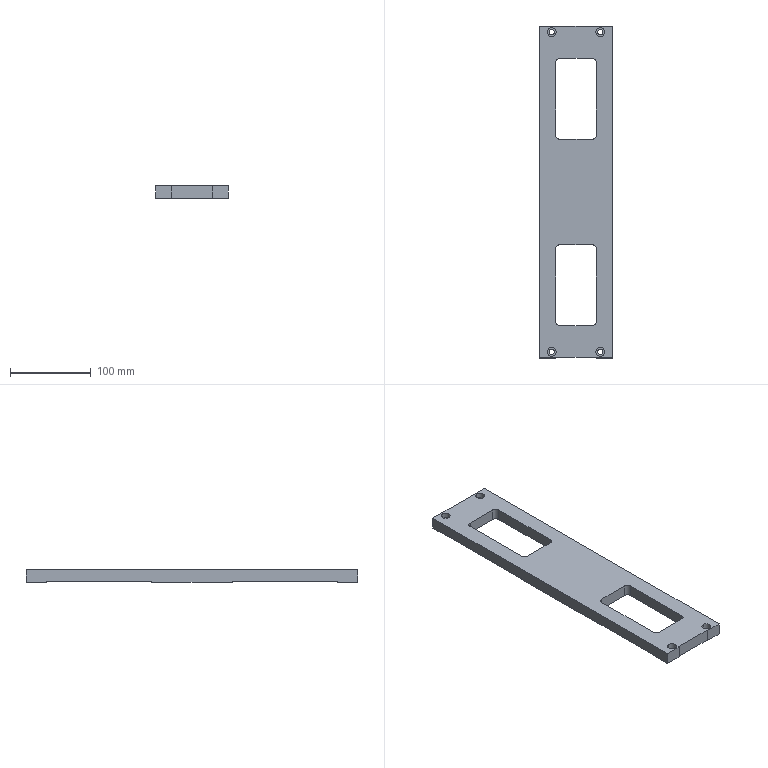NC program | NX | posted with a generic post | part box 90 x 410 x 15 mm
Lines 3599 to 4348 of 4348:
(CAVITY_MILL_COPY_1_COPY , TOOL : D10JING)
N7166 T11 M6
N7168 G54
N7170 G17 G0 G90 X-157.536 Y-18. S9500 M3
N7172 G43 Z30. H11
N7174 Z-14.
N7176 G94 G1 Z-15. F1000.
N7178 X-159.5 Y-19.134
N7180 G3 X-160. Y-20. R1.
N7182 G1 X-70. F1200.
N7184 Y20.
N7186 X-160.
N7188 Y-20.
N7190 G3 X-159.134 Y-19.5 R1.
N7192 G1 X-158. Y-17.536
N7194 Z-14.
N7196 G0 Z30.
N7198 X157.536 Y18.
N7200 Z-14.
N7202 G1 Z-15. F1000.
N7204 X159.5 Y19.134
N7206 G3 X160. Y20. R1.
N7208 G1 X70. F1200.
N7210 Y-20.
N7212 X160.
N7214 Y20.
N7216 G3 X159.134 Y19.5 R1.
N7218 G1 X158. Y17.536
N7220 Z-14.
N7222 G0 Z30.
N7224 M5
(FLOOR_WALL_COPY , TOOL : D10)
N7226 T10 M6
N7228 G54
N7230 G17 G0 G90 X-173.997 Y-51.5 S9500 M3
N7232 G43 Z30. H10
N7234 Z1.
N7236 G94 G1 Z-0.5 F1000.
N7238 Y-49.134
N7240 G3 X-174.497 Y-50. R1.
N7242 G1 Y50. F1200.
N7244 X-169.539
N7246 Y-50.
N7248 X-164.581
N7250 Y50.
N7252 X-159.622
N7254 Y-50.
N7256 X-154.664
N7258 Y50.
N7260 X-149.706
N7262 Y-50.
N7264 X-144.748
N7266 Y50.
N7268 X-139.79
N7270 Y-50.
N7272 X-134.831
N7274 Y50.
N7276 X-129.873
N7278 Y-50.
N7280 X-124.915
N7282 Y50.
N7284 X-119.957
N7286 Y-50.
N7288 X-114.999
N7290 Y50.
N7292 X-110.04
N7294 Y-50.
N7296 X-105.082
N7298 Y50.
N7300 X-100.124
N7302 Y-50.
N7304 X-95.166
N7306 Y50.
N7308 X-90.207
N7310 Y-50.
N7312 X-85.249
N7314 Y50.
N7316 X-80.291
N7318 Y-50.
N7320 X-75.333
N7322 Y50.
N7324 X-70.375
N7326 Y-50.
N7328 X-65.416
N7330 Y50.
N7332 X-60.458
N7334 Y-50.
N7336 X-55.5
N7338 Y50.
N7340 G3 X-56. Y50.866 R1.
N7342 G1 X-57.098 Y51.5
N7344 Z1.
N7346 G0 X-56.598 Y-51.5
N7348 G1 Z-0.5 F1000.
N7350 X-55.5 Y-50.866
N7352 G3 X-55. Y-50. R1.
N7354 G1 Y50. F1200.
N7356 G3 X-55.5 Y50.866 R1.
N7358 G1 X-56.598 Y51.5
N7360 Z1.
N7362 G0 X-173.402
N7364 G1 Z-0.5 F1000.
N7366 X-174.5 Y50.866
N7368 G3 X-175. Y50. R1.
N7370 G1 Y-50. F1200.
N7372 G3 X-174.5 Y-50.866 R1.
N7374 G1 X-173.402 Y-51.5
N7376 Z1.
N7378 G0 Z30.
N7380 X56.003
N7382 Z1.
N7384 G1 Z-0.5 F1000.
N7386 Y-49.134
N7388 G3 X55.503 Y-50. R1.
N7390 G1 Y50. F1200.
N7392 X60.461
N7394 Y-50.
N7396 X65.419
N7398 Y50.
N7400 X70.378
N7402 Y-50.
N7404 X75.336
N7406 Y50.
N7408 X80.294
N7410 Y-50.
N7412 X85.252
N7414 Y50.
N7416 X90.21
N7418 Y-50.
N7420 X95.169
N7422 Y50.
N7424 X100.127
N7426 Y-50.
N7428 X105.085
N7430 Y50.
N7432 X110.043
N7434 Y-50.
N7436 X115.001
N7438 Y50.
N7440 X119.96
N7442 Y-50.
N7444 X124.918
N7446 Y50.
N7448 X129.876
N7450 Y-50.
N7452 X134.834
N7454 Y50.
N7456 X139.793
N7458 Y-50.
N7460 X144.751
N7462 Y50.
N7464 X149.709
N7466 Y-50.
N7468 X154.667
N7470 Y50.
N7472 X159.625
N7474 Y-50.
N7476 X164.584
N7478 Y50.
N7480 X169.542
N7482 Y-50.
N7484 X174.5
N7486 Y50.
N7488 G3 X174. Y50.866 R1.
N7490 G1 X172.902 Y51.5
N7492 Z1.
N7494 G0 X173.402 Y-51.5
N7496 G1 Z-0.5 F1000.
N7498 X174.5 Y-50.866
N7500 G3 X175. Y-50. R1.
N7502 G1 Y50. F1200.
N7504 G3 X174.5 Y50.866 R1.
N7506 G1 X173.402 Y51.5
N7508 Z1.
N7510 G0 X56.598
N7512 G1 Z-0.5 F1000.
N7514 X55.5 Y50.866
N7516 G3 X55. Y50. R1.
N7518 G1 Y-50. F1200.
N7520 G3 X55.5 Y-50.866 R1.
N7522 G1 X56.598 Y-51.5
N7524 Z1.
N7526 G0 Z30.
N7528 M5
(HOLE_MILLING , TOOL : D4)
N7530 T04 M6
N7532 G54
N7534 G17 G0 G90 X-198.5 Y0. S9500 M3
N7536 G43 Z30. H4
N7538 Z0.5
N7540 G94 G3 X-198.95 Y-0.45 R0.45 F1500.
N7542 X-198.5 Y-0.9 R0.45
N7544 X-198.5 Y-0.9 Z0.25 I0. J0.9
N7546 X-198.5 Y-0.9 Z0. I0. J0.9
N7548 X-198.5 Y-0.9 Z-0.25 I0. J0.9
N7550 X-198.5 Y-0.9 Z-0.5 I0. J0.9
N7552 X-198.5 Y-0.9 Z-0.75 I0. J0.9
N7554 X-198.5 Y-0.9 Z-1. I0. J0.9
N7556 X-198.5 Y-0.9 Z-1.25 I0. J0.9
N7558 X-198.5 Y-0.9 Z-1.5 I0. J0.9
N7560 X-198.5 Y-0.9 Z-1.75 I0. J0.9
N7562 X-198.5 Y-0.9 Z-2. I0. J0.9
N7564 X-198.5 Y-0.9 Z-2.25 I0. J0.9
N7566 X-198.5 Y-0.9 Z-2.5 I0. J0.9
N7568 X-198.5 Y-0.9 Z-2.75 I0. J0.9
N7570 X-198.5 Y-0.9 Z-3. I0. J0.9
N7572 X-198.5 Y-0.9 Z-3.25 I0. J0.9
N7574 X-198.5 Y-0.9 Z-3.5 I0. J0.9
N7576 X-198.5 Y-0.9 Z-3.75 I0. J0.9
N7578 X-198.5 Y-0.9 Z-4. I0. J0.9
N7580 X-198.5 Y-0.9 Z-4.25 I0. J0.9
N7582 X-198.5 Y-0.9 Z-4.5 I0. J0.9
N7584 X-198.5 Y-0.9 Z-4.75 I0. J0.9
N7586 X-198.5 Y-0.9 Z-5. I0. J0.9
N7588 X-198.5 Y-0.9 Z-5.25 I0. J0.9
N7590 X-198.5 Y-0.9 Z-5.5 I0. J0.9
N7592 X-198.5 Y-0.9 Z-5.75 I0. J0.9
N7594 X-198.5 Y-0.9 Z-6. I0. J0.9
N7596 X-198.5 Y-0.9 Z-6.25 I0. J0.9
N7598 X-198.5 Y-0.9 Z-6.5 I0. J0.9
N7600 X-198.5 Y-0.9 Z-6.75 I0. J0.9
N7602 X-198.5 Y-0.9 Z-7. I0. J0.9
N7604 X-198.5 Y-0.9 Z-7.25 I0. J0.9
N7606 X-198.5 Y-0.9 Z-7.5 I0. J0.9
N7608 X-198.5 Y-0.9 Z-7.75 I0. J0.9
N7610 X-198.5 Y-0.9 Z-8. I0. J0.9
N7612 X-197.6 Y0. R0.9
N7614 X-198.5 Y-0.9 R-0.9
N7616 X-198.05 Y-0.45 R0.45
N7618 X-198.5 Y0. R0.45
N7620 G0 Z30.
N7622 X197.5
N7624 Z0.5
N7626 G3 X197.05 Y-0.45 R0.45
N7628 X197.5 Y-0.9 R0.45
N7630 X197.5 Y-0.9 Z0.25 I0. J0.9
N7632 X197.5 Y-0.9 Z0. I0. J0.9
N7634 X197.5 Y-0.9 Z-0.25 I0. J0.9
N7636 X197.5 Y-0.9 Z-0.5 I0. J0.9
N7638 X197.5 Y-0.9 Z-0.75 I0. J0.9
N7640 X197.5 Y-0.9 Z-1. I0. J0.9
N7642 X197.5 Y-0.9 Z-1.25 I0. J0.9
N7644 X197.5 Y-0.9 Z-1.5 I0. J0.9
N7646 X197.5 Y-0.9 Z-1.75 I0. J0.9
N7648 X197.5 Y-0.9 Z-2. I0. J0.9
N7650 X197.5 Y-0.9 Z-2.25 I0. J0.9
N7652 X197.5 Y-0.9 Z-2.5 I0. J0.9
N7654 X197.5 Y-0.9 Z-2.75 I0. J0.9
N7656 X197.5 Y-0.9 Z-3. I0. J0.9
N7658 X197.5 Y-0.9 Z-3.25 I0. J0.9
N7660 X197.5 Y-0.9 Z-3.5 I0. J0.9
N7662 X197.5 Y-0.9 Z-3.75 I0. J0.9
N7664 X197.5 Y-0.9 Z-4. I0. J0.9
N7666 X197.5 Y-0.9 Z-4.25 I0. J0.9
N7668 X197.5 Y-0.9 Z-4.5 I0. J0.9
N7670 X197.5 Y-0.9 Z-4.75 I0. J0.9
N7672 X197.5 Y-0.9 Z-5. I0. J0.9
N7674 X197.5 Y-0.9 Z-5.25 I0. J0.9
N7676 X197.5 Y-0.9 Z-5.5 I0. J0.9
N7678 X197.5 Y-0.9 Z-5.75 I0. J0.9
N7680 X197.5 Y-0.9 Z-6. I0. J0.9
N7682 X197.5 Y-0.9 Z-6.25 I0. J0.9
N7684 X197.5 Y-0.9 Z-6.5 I0. J0.9
N7686 X197.5 Y-0.9 Z-6.75 I0. J0.9
N7688 X197.5 Y-0.9 Z-7. I0. J0.9
N7690 X197.5 Y-0.9 Z-7.25 I0. J0.9
N7692 X197.5 Y-0.9 Z-7.5 I0. J0.9
N7694 X197.5 Y-0.9 Z-7.75 I0. J0.9
N7696 X197.5 Y-0.9 Z-8. I0. J0.9
N7698 X198.4 Y0. R0.9
N7700 X197.5 Y-0.9 R-0.9
N7702 X197.95 Y-0.45 R0.45
N7704 X197.5 Y0. R0.45
N7706 G0 Z30.
N7708 M5
(PLANAR_MILL_1 , TOOL : D6A45)
N7710 T07 M6
N7712 G54
N7714 G17 G0 G90 X198.592 Y-30.498 S9500 M3
N7716 G43 Z30. H7
N7718 Z0.5
N7720 G94 G1 Z-1. F1250.
N7722 X199.4 Y-30.866
N7724 G3 X199.9 Y-30. R1.
N7726 X197.5 Y-27.6 R2.4
N7728 X199.9 Y-30. R-2.4
N7730 X199.4 Y-29.134 R1.
N7732 G1 X198.592 Y-29.502
N7734 Z0.5
N7736 G0 Z30.
N7738 X198.291 Y-0.428
N7740 Z0.5
N7742 G1 Z-1.
N7744 X199.1 Y-0.866
N7746 G3 X199.6 Y0. R1.
N7748 X197.5 Y2.1 R2.1
N7750 X199.6 Y0. R-2.1
N7752 X199.1 Y0.866 R1.
N7754 G1 X198.291 Y0.428
N7756 Z0.5
N7758 G0 Z30.
N7760 X198.592 Y29.502
N7762 Z0.5
N7764 G1 Z-1.
N7766 X199.4 Y29.134
N7768 G3 X199.9 Y30. R1.
N7770 X197.5 Y32.4 R2.4
N7772 X199.9 Y30. R-2.4
N7774 X199.4 Y30.866 R1.
N7776 G1 X198.592 Y30.498
N7778 Z0.5
N7780 G0 Z30.
N7782 X37.437 Y39.825
N7784 Z0.5
N7786 G1 X37.4 Y39.759 Z0.48
N7788 Y39.5 Z0.41
N7790 Y39.241 Z0.341
N7792 X37.701 Y38.701 Z0.175
N7794 X38.241 Y38.4 Z0.009
N7796 X38.759 Z-0.129
N7798 X39.299 Y38.701 Z-0.295
N7800 X39.6 Y39.241 Z-0.461
N7802 Y39.759 Z-0.599
N7804 X39.299 Y40.299 Z-0.765
N7806 X38.759 Y40.6 Z-0.931
N7808 X38.5 Z-1.
N7810 G3 X37.4 Y39.5 R1.1
N7812 X38.5 Y40.6 R-1.1
N7814 X37.634 Y40.1 R1.
N7816 G1 Z0.5
N7818 G0 Z30.
N7820 X39.126 Y25.424
N7822 Z0.5
N7824 G1 X39.052 Y25.552 Z0.46
N7826 X38.714 Y25.75 Z0.356
N7828 X38.286 Z0.241
N7830 X37.948 Y25.552 Z0.136
N7832 X37.75 Y25.214 Z0.031
N7834 Y24.786 Z-0.084
N7836 X37.948 Y24.448 Z-0.189
N7838 X38.286 Y24.25 Z-0.294
N7840 X38.714 Z-0.408
N7842 X39.052 Y24.448 Z-0.513
N7844 X39.25 Y24.786 Z-0.618
N7846 Y25.214 Z-0.733
N7848 X39.052 Y25.552 Z-0.838
N7850 X38.714 Y25.75 Z-0.943
N7852 X38.5 Z-1.
N7854 G3 X37.75 Y25. R0.75
N7856 X38.5 Y25.75 R-0.75
N7858 X38.067 Y25.5 R0.5
N7860 G1 Z0.5
N7862 G0 Z30.
N7864 X37.437 Y0.325
N7866 Z0.5
N7868 G1 X37.4 Y0.259 Z0.48
N7870 Y0. Z0.41
N7872 Y-0.259 Z0.341
N7874 X37.701 Y-0.799 Z0.175
N7876 X38.241 Y-1.1 Z0.009
N7878 X38.759 Z-0.129
N7880 X39.299 Y-0.799 Z-0.295
N7882 X39.6 Y-0.259 Z-0.461
N7884 Y0.259 Z-0.599
N7886 X39.299 Y0.799 Z-0.765
N7888 X38.759 Y1.1 Z-0.931
N7890 X38.5 Z-1.
N7892 G3 X37.4 Y0. R1.1
N7894 X38.5 Y1.1 R-1.1
N7896 X37.634 Y0.6 R1.
N7898 G1 Z0.5
N7900 G0 Z30.
N7902 X37.874 Y-25.424
N7904 Z0.5
N7906 G1 X37.948 Y-25.552 Z0.46
N7908 X38.286 Y-25.75 Z0.356
N7910 X38.714 Z0.241
N7912 X39.052 Y-25.552 Z0.136
N7914 X39.25 Y-25.214 Z0.031
N7916 Y-24.786 Z-0.084
N7918 X39.052 Y-24.448 Z-0.189
N7920 X38.714 Y-24.25 Z-0.294
N7922 X38.286 Z-0.408
N7924 X37.948 Y-24.448 Z-0.513
N7926 X37.75 Y-24.786 Z-0.618
N7928 Y-25.214 Z-0.733
N7930 X37.948 Y-25.552 Z-0.838
N7932 X38.286 Y-25.75 Z-0.943
N7934 X38.5 Z-1.
N7936 G3 X39.25 Y-25. R0.75
N7938 X38.5 Y-25.75 R-0.75
N7940 X38.933 Y-25.5 R0.5
N7942 G1 Z0.5
N7944 G0 Z30.
N7946 X48.714 Y-47.374
N7948 Z0.5
N7950 G1 Z-1.
N7952 X48.92 Y-46.893
N7954 G3 X48.8 Y-45.9 R1.
N7956 G1 X-48.8
N7958 G3 X-48.92 Y-46.893 R1.
N7960 G1 X-48.714 Y-47.374
N7962 Z0.5
N7964 G0 Z30.
N7966 X-181.286
N7968 Z0.5
N7970 G1 Z-1.
N7972 X-181.08 Y-46.893
N7974 G3 X-181.2 Y-45.9 R1.
N7976 G1 X-204.9
N7978 G2 X-205.9 Y-44.9 R1.
N7980 G1 Y44.9
N7982 G2 X-204.9 Y45.9 R1.
N7984 G1 X-181.2
N7986 G3 X-181.08 Y46.893 R1.
N7988 G1 X-181.286 Y47.374
N7990 Z0.5
N7992 G0 Z30.
N7994 X-48.714
N7996 Z0.5
N7998 G1 Z-1.
N8000 X-48.92 Y46.893
N8002 G3 X-48.8 Y45.9 R1.
N8004 G1 X48.8
N8006 G3 X48.92 Y46.893 R1.
N8008 G1 X48.714 Y47.374
N8010 Z0.5
N8012 G0 Z30.
N8014 X181.286
N8016 Z0.5
N8018 G1 Z-1.
N8020 X181.08 Y46.893
N8022 G3 X181.2 Y45.9 R1.
N8024 G1 X204.9
N8026 G2 X205.9 Y44.9 R1.
N8028 G1 Y25.1
N8030 G2 X204.9 Y24.1 R1.
N8032 G1 Y-24.1
N8034 G2 X205.9 Y-25.1 R1.
N8036 G1 Y-44.9
N8038 G2 X204.9 Y-45.9 R1.
N8040 G1 X181.2
N8042 G3 X181.08 Y-46.893 R1.
N8044 G1 X181.286 Y-47.374
N8046 Z0.5
N8048 G0 Z30.
N8050 X-39.126 Y-25.424
N8052 Z0.5
N8054 G1 X-39.052 Y-25.552 Z0.46
N8056 X-38.714 Y-25.75 Z0.356
N8058 X-38.286 Z0.241
N8060 X-37.948 Y-25.552 Z0.136
N8062 X-37.75 Y-25.214 Z0.031
N8064 Y-24.786 Z-0.084
N8066 X-37.948 Y-24.448 Z-0.189
N8068 X-38.286 Y-24.25 Z-0.294
N8070 X-38.714 Z-0.408
N8072 X-39.052 Y-24.448 Z-0.513
N8074 X-39.25 Y-24.786 Z-0.618
N8076 Y-25.214 Z-0.733
N8078 X-39.052 Y-25.552 Z-0.838
N8080 X-38.714 Y-25.75 Z-0.943
N8082 X-38.5 Z-1.
N8084 G3 X-37.75 Y-25. R0.75
N8086 X-38.5 Y-25.75 R-0.75
N8088 X-38.067 Y-25.5 R0.5
N8090 G1 Z0.5
N8092 G0 Z30.
N8094 X-37.437 Y-0.325
N8096 Z0.5
N8098 G1 X-37.4 Y-0.259 Z0.48
N8100 Y0. Z0.41
N8102 Y0.259 Z0.341
N8104 X-37.701 Y0.799 Z0.175
N8106 X-38.241 Y1.1 Z0.009
N8108 X-38.759 Z-0.129
N8110 X-39.299 Y0.799 Z-0.295
N8112 X-39.6 Y0.259 Z-0.461
N8114 Y-0.259 Z-0.599
N8116 X-39.299 Y-0.799 Z-0.765
N8118 X-38.759 Y-1.1 Z-0.931
N8120 X-38.5 Z-1.
N8122 G3 X-37.4 Y0. R1.1
N8124 X-38.5 Y-1.1 R-1.1
N8126 X-37.634 Y-0.6 R1.
N8128 G1 Z0.5
N8130 G0 Z30.
N8132 X-37.874 Y25.424
N8134 Z0.5
N8136 G1 X-37.948 Y25.552 Z0.46
N8138 X-38.286 Y25.75 Z0.356
N8140 X-38.714 Z0.241
N8142 X-39.052 Y25.552 Z0.136
N8144 X-39.25 Y25.214 Z0.031
N8146 Y24.786 Z-0.084
N8148 X-39.052 Y24.448 Z-0.189
N8150 X-38.714 Y24.25 Z-0.294
N8152 X-38.286 Z-0.408
N8154 X-37.948 Y24.448 Z-0.513
N8156 X-37.75 Y24.786 Z-0.618
N8158 Y25.214 Z-0.733
N8160 X-37.948 Y25.552 Z-0.838
N8162 X-38.286 Y25.75 Z-0.943
N8164 X-38.5 Z-1.
N8166 G3 X-39.25 Y25. R0.75
N8168 X-38.5 Y25.75 R-0.75
N8170 X-38.933 Y25.5 R0.5
N8172 G1 Z0.5
N8174 G0 Z30.
N8176 X-39.563 Y39.825
N8178 Z0.5
N8180 G1 X-39.6 Y39.759 Z0.48
N8182 Y39.5 Z0.41
N8184 Y39.241 Z0.341
N8186 X-39.299 Y38.701 Z0.175
N8188 X-38.759 Y38.4 Z0.009
N8190 X-38.241 Z-0.129
N8192 X-37.701 Y38.701 Z-0.295
N8194 X-37.4 Y39.241 Z-0.461
N8196 Y39.759 Z-0.599
N8198 X-37.701 Y40.299 Z-0.765
N8200 X-38.241 Y40.6 Z-0.931
N8202 X-38.5 Z-1.
N8204 G3 X-39.6 Y39.5 R1.1
N8206 X-38.5 Y40.6 R-1.1
N8208 X-39.366 Y40.1 R1.
N8210 G1 Z0.5
N8212 G0 Z30.
N8214 X-198.592 Y30.498
N8216 Z0.5
N8218 G1 Z-1.
N8220 X-199.4 Y30.866
N8222 G3 X-199.9 Y30. R1.
N8224 X-197.5 Y27.6 R2.4
N8226 X-199.9 Y30. R-2.4
N8228 X-199.4 Y29.134 R1.
N8230 G1 X-198.592 Y29.502
N8232 Z0.5
N8234 G0 Z30.
N8236 X-199.291 Y0.428
N8238 Z0.5
N8240 G1 Z-1.
N8242 X-200.1 Y0.866
N8244 G3 X-200.6 Y0. R1.
N8246 X-198.5 Y-2.1 R2.1
N8248 X-200.6 Y0. R-2.1
N8250 X-200.1 Y-0.866 R1.
N8252 G1 X-199.291 Y-0.428
N8254 Z0.5
N8256 G0 Z30.
N8258 X-198.592 Y-29.502
N8260 Z0.5
N8262 G1 Z-1.
N8264 X-199.4 Y-29.134
N8266 G3 X-199.9 Y-30. R1.
N8268 X-197.5 Y-32.4 R2.4
N8270 X-199.9 Y-30. R-2.4
N8272 X-199.4 Y-30.866 R1.
N8274 G1 X-198.592 Y-30.498
N8276 Z0.5
N8278 G0 Z30.
(PLANAR_MILL_1_COPY , TOOL : D6A45)
N8280 X113.73 Y-23.4
N8282 Z0.5
N8284 G1 Z-1.
N8286 X114.134 Y-24.1
N8288 G3 X115. Y-24.6 R1.
N8290 G1 X160.
N8292 G3 X164.6 Y-20. R4.6
N8294 G1 Y20.
N8296 G3 X160. Y24.6 R4.6
N8298 G1 X70.
N8300 G3 X65.4 Y20. R4.6
N8302 G1 Y-20.
N8304 G3 X70. Y-24.6 R4.6
N8306 G1 X115.
N8308 G3 X115.866 Y-24.1 R1.
N8310 G1 X116.27 Y-23.4
N8312 Z0.5
N8314 G0 Z30.
N8316 X177.936 Y-46.741
N8318 Z0.5
N8320 G1 Z-1.
N8322 X178.303 Y-46.368
N8324 G3 X178.554 Y-45.4 R1.
N8326 G1 X51.446
N8328 G3 X51.697 Y-46.368 R1.
N8330 G1 X52.064 Y-46.741
N8332 Z0.5
N8334 G0 Z30.
N8336 X-52.064
N8338 Z0.5
N8340 G1 Z-1.
N8342 X-51.697 Y-46.368
N8344 G3 X-51.446 Y-45.4 R1.
N8346 G1 X-178.554
N8348 G3 X-178.303 Y-46.368 R1.
N8350 G1 X-177.936 Y-46.741
N8352 Z0.5
N8354 G0 Z30.
N8356 Y46.741
N8358 Z0.5
N8360 G1 Z-1.
N8362 X-178.303 Y46.368
N8364 G3 X-178.554 Y45.4 R1.
N8366 G1 X-51.446
N8368 G3 X-51.697 Y46.368 R1.
N8370 G1 X-52.064 Y46.741
N8372 Z0.5
N8374 G0 Z30.
N8376 X52.064
N8378 Z0.5
N8380 G1 Z-1.
N8382 X51.697 Y46.368
N8384 G3 X51.446 Y45.4 R1.
N8386 G1 X178.554
N8388 G3 X178.303 Y46.368 R1.
N8390 G1 X177.936 Y46.741
N8392 Z0.5
N8394 G0 Z30.
N8396 X-113.73 Y23.4
N8398 Z0.5
N8400 G1 Z-1.
N8402 X-114.134 Y24.1
N8404 G3 X-115. Y24.6 R1.
N8406 G1 X-160.
N8408 G3 X-164.6 Y20. R4.6
N8410 G1 Y-20.
N8412 G3 X-160. Y-24.6 R4.6
N8414 G1 X-70.
N8416 G3 X-65.4 Y-20. R4.6
N8418 G1 Y20.
N8420 G3 X-70. Y24.6 R4.6
N8422 G1 X-115.
N8424 G3 X-115.866 Y24.1 R1.
N8426 G1 X-116.27 Y23.4
N8428 Z0.5
N8430 G0 Z30.
N8432 M5
(刀补4 , TOOL : D4)
N8434 T04 M6
N8436 G54
N8438 G17 G0 G90 X-198.5 Y0. S9500 M3
N8440 G43 Z30. H4
N8442 Z0.5
N8444 G41 G94 G1 X-198.6 Y-0.004 F1500. D4
N8446 G3 X-198.5 Y-0.95 R0.478
N8448 X-198.5 Y-0.95 Z-1.5 I0. J0.95
N8450 X-198.5 Y-0.95 Z-3.5 I0. J0.95
N8452 X-198.5 Y-0.95 Z-5.5 I0. J0.95
N8454 X-198.5 Y-0.95 Z-7.5 I0. J0.95
N8456 X-197.55 Y0. Z-8. R0.95
N8458 X-198.5 Y0.95 R0.95
N8460 X-197.55 Y0. R-0.95
N8462 X-198.496 Y0.1 R0.478
N8464 G40
N8466 G1 X-198.5 Y0.
N8468 G0 Z30.
N8470 X197.5
N8472 Z0.5
N8474 G41 G1 X197.4 Y-0.004
N8476 G3 X197.5 Y-0.95 R0.478
N8478 X197.5 Y-0.95 Z-1.5 I0. J0.95
N8480 X197.5 Y-0.95 Z-3.5 I0. J0.95
N8482 X197.5 Y-0.95 Z-5.5 I0. J0.95
N8484 X197.5 Y-0.95 Z-7.5 I0. J0.95
N8486 X198.45 Y0. Z-8. R0.95
N8488 X197.5 Y0.95 R0.95
N8490 X198.45 Y0. R-0.95
N8492 X197.504 Y0.1 R0.478
N8494 G40
N8496 G1 X197.5 Y0.
N8498 G0 Z30.
N8500 M5
(刀补3 , TOOL : D3)
N8502 T03 M6
N8504 G54
N8506 G17 G0 G90 X-38.5 Y39.5 S9500 M3
N8508 G43 Z30. H3
N8510 Z0.5
N8512 G41 G94 G1 X-38.596 Y39.473 F1200. D3
N8514 G3 X-38.5 Y39.05 R0.222
N8516 X-38.5 Y39.05 Z-1.5 I0. J0.45
N8518 X-38.5 Y39.05 Z-3.5 I0. J0.45
N8520 X-38.5 Y39.05 Z-5.5 I0. J0.45
N8522 X-38.05 Y39.5 Z-6. R0.45
N8524 X-38.5 Y39.95 R0.45
N8526 X-38.05 Y39.5 R-0.45
N8528 X-38.473 Y39.596 R0.222
N8530 G40
N8532 G1 X-38.5 Y39.5
N8534 G0 Z30.
N8536 Y0.
N8538 Z0.5
N8540 G41 G1 X-38.596 Y-0.027
N8542 G3 X-38.5 Y-0.45 R0.222
N8544 X-38.5 Y-0.45 Z-1.5 I0. J0.45
N8546 X-38.5 Y-0.45 Z-3.5 I0. J0.45
N8548 X-38.5 Y-0.45 Z-5.5 I0. J0.45
N8550 X-38.05 Y0. Z-6. R0.45
N8552 X-38.5 Y0.45 R0.45
N8554 X-38.05 Y0. R-0.45
N8556 X-38.473 Y0.096 R0.222
N8558 G40
N8560 G1 X-38.5 Y0.
N8562 G0 Z30.
N8564 X38.5 Y39.5
N8566 Z0.5
N8568 G41 G1 X38.404 Y39.473
N8570 G3 X38.5 Y39.05 R0.222
N8572 X38.5 Y39.05 Z-1.5 I0. J0.45
N8574 X38.5 Y39.05 Z-3.5 I0. J0.45
N8576 X38.5 Y39.05 Z-5.5 I0. J0.45
N8578 X38.95 Y39.5 Z-6. R0.45
N8580 X38.5 Y39.95 R0.45
N8582 X38.95 Y39.5 R-0.45
N8584 X38.527 Y39.596 R0.222
N8586 G40
N8588 G1 X38.5 Y39.5
N8590 G0 Z30.
N8592 Y0.
N8594 Z0.5
N8596 G41 G1 X38.404 Y-0.027
N8598 G3 X38.5 Y-0.45 R0.222
N8600 X38.5 Y-0.45 Z-1.5 I0. J0.45
N8602 X38.5 Y-0.45 Z-3.5 I0. J0.45
N8604 X38.5 Y-0.45 Z-5.5 I0. J0.45
N8606 X38.95 Y0. Z-6. R0.45
N8608 X38.5 Y0.45 R0.45
N8610 X38.95 Y0. R-0.45
N8612 X38.527 Y0.096 R0.222
N8614 G40
N8616 G1 X38.5 Y0.
N8618 G0 Z30.
N8620 M5
N8622 M2